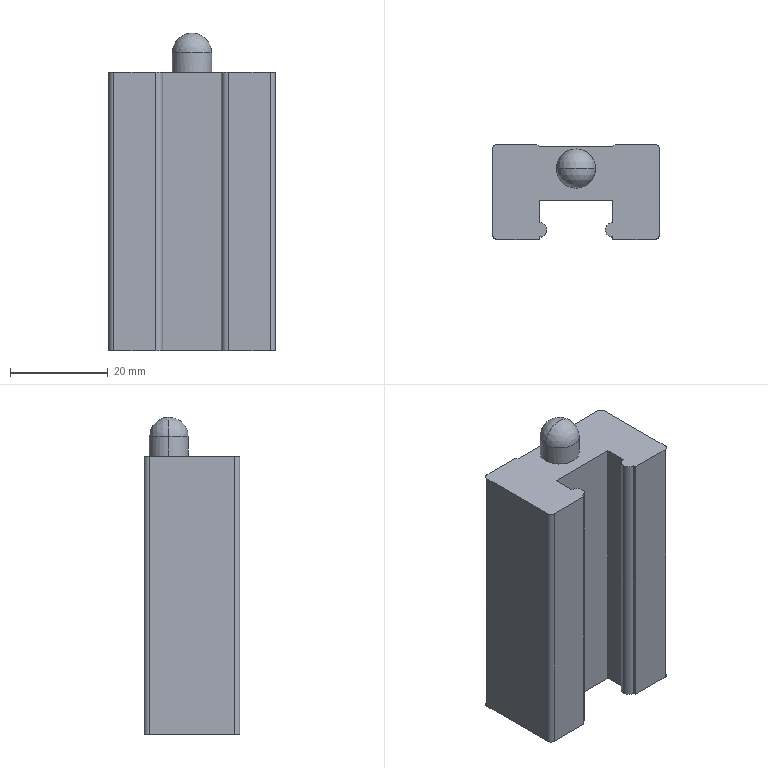Part | STEP file | Slider 15_THK_SSR15XW | 1 solid | 63 faces | box 34 x 19.5 x 65 mm | volume 30926 mm3 | cylinder 25 | plane 20 | cone 16 | sphere 2 | commonest cylinder face diameters 3.2 x8 3.3 x8 2 x4 3 x3 8 x2